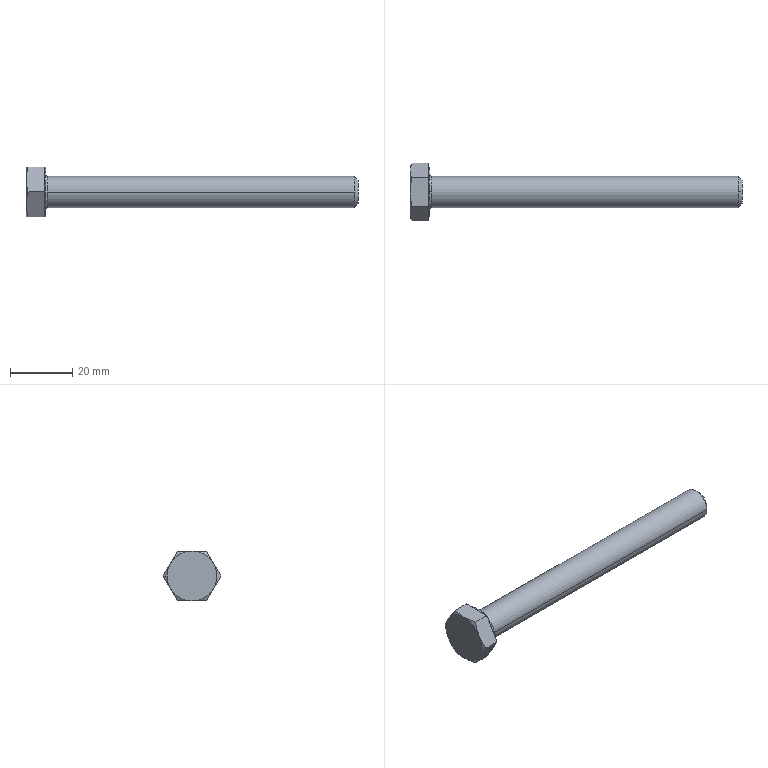Part | STEP file | 1 solid | 37 faces | box 106.4 x 18.475 x 16 mm | volume 9236 mm3 | cone 16 | plane 15 | cylinder 4 | spline 2 | commonest cylinder face diameters 10 x2 16 x2